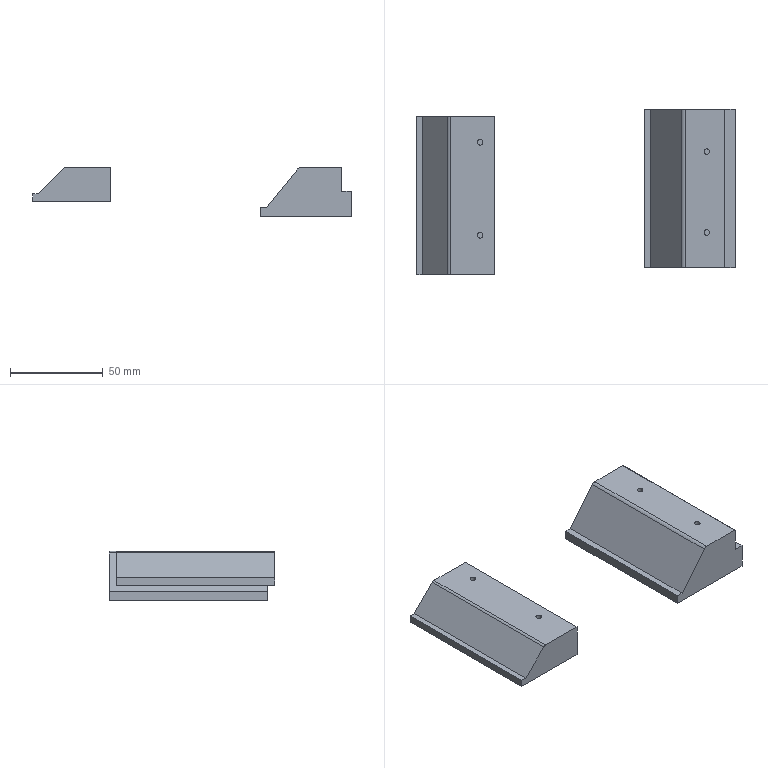NC program | NX | posted with a generic post | part box 171.319 x 88.841 x 26.598 mm
Lines 985 to 3096 of 3096, first 1925 of 2100 lines:
(ZLEVEL_PROFILE_COPY , TOOL : D6R0.5)
N1950 T16 M6
N1952 G54
N1954 G17 G0 G90 X44.509 Y-6.044 S9500 M3
N1956 G43 Z30. H16
N1958 Z1.492
N1960 G94 G1 Z-0.008 F1000.
N1962 X44.022 Y-5.216
N1964 G3 X43.5 Y-4.92 R0.6
N1966 G1 X43.356 Y-4.921 F3000.
N1968 X42.5 Y-5.121
N1970 X-42.5
N1972 X-43.237 Y-4.931
N1974 G2 X-43.39 Y-5.022 R0.113
N1976 G1 X-43.445 Y-5.
N1978 X-43.502 Y-4.969
N1980 X-43.5 Y-5.065 Z-0.017
N1982 G3 X-42.5 Y-5.216 R13.441
N1984 G1 X42.5
N1986 G3 X43.5 Y-5.028 R4.279
N1988 G1 Y-5.14 Z-0.026
N1990 G2 X42.5 Y-5.29 R40.754
N1992 G1 X-42.5
N1994 G2 X-43.5 Y-5.126 R8.99
N1996 G1 Y-5.185 Z-0.035
N1998 G3 X-42.5 Y-5.354 R10.525
N2000 G1 X42.5
N2002 G3 X43.5 Y-5.198 R68.272
N2004 G1 Y-5.242 Z-0.04
N2006 Y-5.252 Z-0.045
N2008 G2 X42.5 Y-5.42 R6.122
N2010 G1 X-42.5
N2012 G2 X-43.5 Y-5.233 R5.293
N2014 G1 Y-5.299 Z-0.06
N2016 G3 X-42.5 Y-5.499 R12.388
N2018 G1 X42.5
N2020 X43.5 Y-5.326
N2022 Y-5.392 Z-0.069
N2024 Y-5.412 Z-0.078
N2026 X42.5 Y-5.579
N2028 X-42.5
N2030 G2 X-43.5 Y-5.378 R2.866
N2032 G1 Y-5.468 Z-0.098
N2034 X-43.376 Y-5.509
N2036 X-42.5 Y-5.659
N2038 X42.5
N2040 X43.5 Y-5.51
N2042 Y-5.548 Z-0.109
N2044 Y-5.585 Z-0.121
N2046 X42.5 Y-5.742
N2048 X-42.5
N2050 X-42.665 Y-5.718
N2052 X-43.529 Y-5.568
N2054 Y-5.602 Z-0.134
N2056 Y-5.658 Z-0.147
N2058 X-42.665 Y-5.813
N2060 X-42.5 Y-5.826
N2062 X42.5
N2064 X43.5 Y-5.67
N2066 Y-5.72 Z-0.161
N2068 Y-5.765 Z-0.175
N2070 X42.5 Y-5.911
N2072 X-42.5
N2074 X-42.665 Y-5.898
N2076 X-43.529 Y-5.758
N2078 X-43.5 Y-5.864 Z-0.207
N2080 X-42.5 Y-5.995
N2082 X42.5
N2084 X43.5 Y-5.866
N2086 Y-5.922 Z-0.224
N2088 Y-5.945 Z-0.242
N2090 X42.5 Y-6.08
N2092 X-42.5
N2094 X-43.5 Y-5.944
N2096 Y-6.008 Z-0.261
N2098 Y-6.031 Z-0.28
N2100 X-43.356 Y-6.034
N2102 X-42.665 Y-6.153
N2104 X-42.5 Y-6.165
N2106 X42.5
N2108 X42.665 Y-6.153
N2110 X43.356 Y-6.035
N2112 X43.5 Y-6.032
N2114 Y-6.092 Z-0.3
N2116 Y-6.126 Z-0.321
N2118 X42.665 Y-6.242
N2120 X42.5 Y-6.249
N2122 X-42.5
N2124 X-42.665 Y-6.242
N2126 X-43.5 Y-6.125
N2128 Y-6.172 Z-0.338
N2130 Y-6.207 Z-0.356
N2132 X-42.665 Y-6.309
N2134 X-42.5 Y-6.317
N2136 X42.5
N2138 X43.5 Y-6.207
N2140 Y-6.251 Z-0.376
N2142 Y-6.289 Z-0.396
N2144 X43.356 Y-6.293
N2146 X42.5 Y-6.389
N2148 X-42.5
N2150 X-42.665 Y-6.383
N2152 X-43.356 Y-6.293
N2154 X-43.5 Y-6.289
N2156 Y-6.342 Z-0.42
N2158 Y-6.387 Z-0.445
N2160 X-43.356 Y-6.389
N2162 X-42.5 Y-6.472
N2164 X42.5
N2166 G2 X43.5 Y-6.387 R24.941
N2168 G1 Y-6.43 Z-0.471
N2170 Y-6.464 Z-0.497
N2172 X43.189 Y-6.47
N2174 X43.011 Y-6.505
N2176 X42.5 Y-6.553
N2178 X-42.5
N2180 G2 X-43.189 Y-6.47 R3.133
N2182 G1 X-43.5 Y-6.464
N2184 Y-6.51 Z-0.524
N2186 Y-6.548 Z-0.551
N2188 X-43.356
N2190 X-42.665 Y-6.625
N2192 X-42.5 Y-6.633
N2194 X42.5
N2196 X42.665 Y-6.625
N2198 X43.356 Y-6.548
N2200 X43.5
N2202 Y-6.588 Z-0.58
N2204 Y-6.625 Z-0.609
N2206 X43.356 Y-6.628
N2208 X42.665 Y-6.706
N2210 X42.5 Y-6.712
N2212 X-42.5
N2214 X-42.665 Y-6.706
N2216 X-43.356 Y-6.628
N2218 X-43.5 Y-6.625
N2220 Y-6.67 Z-0.639
N2222 Y-6.709 Z-0.669
N2224 X-43.356 Y-6.712
N2226 X-42.665 Y-6.781
N2228 X-42.5 Y-6.789
N2230 X42.5
N2232 X42.665 Y-6.781
N2234 X43.356 Y-6.712
N2236 X43.5 Y-6.709
N2238 Y-6.756 Z-0.701
N2240 Y-6.796 Z-0.732
N2242 G3 X42.5 Y-6.864 R11.206
N2244 G1 X-42.5
N2246 X-43.356 Y-6.79
N2248 X-43.5 Y-6.791
N2250 Y-6.834 Z-0.765
N2252 Y-6.868 Z-0.798
N2254 X-43.356 Y-6.87
N2256 X-42.5 Y-6.937
N2258 X42.5
N2260 X43.356 Y-6.872
N2262 X43.5 Y-6.869
N2264 Y-6.907 Z-0.832
N2266 Y-6.936 Z-0.866
N2268 G3 X42.5 Y-7.008 R11.171
N2270 G1 X-42.5
N2272 G3 X-43.5 Y-6.937 R10.417
N2274 G1 Y-6.977 Z-0.901
N2276 Y-7.005 Z-0.936
N2278 X-43.011 Y-7.022
N2280 G3 X-42.5 Y-7.077 R2.311
N2282 G1 X42.5
N2284 G3 X43.011 Y-7.024 R2.413
N2286 G1 X43.5 Y-7.003
N2288 Y-7.043 Z-0.972
N2290 Y-7.072 Z-1.008
N2292 G3 X42.5 Y-7.143 R13.5
N2294 G1 X-42.5
N2296 G3 X-43.5 Y-7.075 R12.04
N2298 G1 Y-7.12 Z-1.045
N2300 Y-7.146 Z-1.083
N2302 G2 X-42.5 Y-7.207 R11.565
N2304 G1 X42.5
N2306 X43.356 Y-7.147
N2308 X43.5 Y-7.142
N2310 Y-7.184 Z-1.121
N2312 Y-7.215 Z-1.159
N2314 X42.5 Y-7.269
N2316 X-42.5
N2318 X-43.356 Y-7.223
N2320 X-43.5 Y-7.22
N2322 Y-7.258 Z-1.198
N2324 Y-7.287 Z-1.237
N2326 G2 X-42.5 Y-7.332 R14.586
N2328 G1 X42.5
N2330 X43.5 Y-7.283
N2332 Y-7.317 Z-1.276
N2334 Y-7.348 Z-1.314
N2336 X42.5 Y-7.395
N2338 X-42.5
N2340 G3 X-43.5 Y-7.353 R13.607
N2342 G1 Y-7.388 Z-1.353
N2344 Y-7.418 Z-1.392
N2346 G2 X-42.5 Y-7.458 R12.751
N2348 G1 X42.5
N2350 X42.665 Y-7.456
N2352 X43.356 Y-7.417
N2354 X43.5 Y-7.413
N2356 Y-7.447 Z-1.431
N2358 Y-7.478 Z-1.47
N2360 X43.356 Y-7.482
N2362 X42.665 Y-7.519
N2364 X42.5 Y-7.521
N2366 X-42.5
N2368 G3 X-43.5 Y-7.483 R11.996
N2370 G1 Y-7.518 Z-1.509
N2372 Y-7.548 Z-1.548
N2374 G2 X-42.5 Y-7.584 R11.325
N2376 G1 X42.5
N2378 X42.665 Y-7.583
N2380 X43.5 Y-7.543
N2382 Y-7.577 Z-1.586
N2384 Y-7.608 Z-1.625
N2386 X43.356 Y-7.613
N2388 X42.665 Y-7.645
N2390 X42.5 Y-7.647
N2392 X-42.5
N2394 G3 X-43.5 Y-7.613 R11.27
N2396 G1 Y-7.648 Z-1.664
N2398 Y-7.678 Z-1.703
N2400 G2 X-42.5 Y-7.71 R12.074
N2402 G1 X42.5
N2404 X42.665 Y-7.708
N2406 X43.5 Y-7.673
N2408 Y-7.708 Z-1.742
N2410 Y-7.739 Z-1.781
N2412 X43.356 Y-7.743
N2414 X42.665 Y-7.771
N2416 X42.5 Y-7.773
N2418 X-42.5
N2420 G3 X-43.5 Y-7.743 R12.986
N2422 G1 Y-7.778 Z-1.82
N2424 Y-7.808 Z-1.858
N2426 G2 X-42.5 Y-7.836 R14.047
N2428 G1 X42.5
N2430 X42.665 Y-7.834
N2432 X43.5 Y-7.804
N2434 Y-7.838 Z-1.897
N2436 Y-7.869 Z-1.936
N2438 X42.665 Y-7.897
N2440 X42.5 Y-7.899
N2442 X-42.5
N2444 G3 X-43.5 Y-7.873 R15.297
N2446 G1 Y-7.909 Z-1.975
N2448 Y-7.938 Z-2.014
N2450 G2 X-42.5 Y-7.962 R16.792
N2452 G1 X42.5
N2454 X42.665 Y-7.96
N2456 X43.5 Y-7.935
N2458 Y-7.968 Z-2.053
N2460 Y-7.999 Z-2.092
N2462 X42.5 Y-8.025
N2464 X-42.5
N2466 X-42.665 Y-8.02
N2468 X-43.5 Y-8.003
N2470 Y-8.039 Z-2.13
N2472 Y-8.068 Z-2.169
N2474 X-42.5 Y-8.087
N2476 X42.5
N2478 X43.5 Y-8.064
N2480 Y-8.098 Z-2.208
N2482 Y-8.129 Z-2.247
N2484 X42.5 Y-8.15
N2486 X-42.5
N2488 X-43.5 Y-8.133
N2490 Y-8.169 Z-2.286
N2492 Y-8.198 Z-2.325
N2494 X-42.5 Y-8.213
N2496 X42.5
N2498 X43.5 Y-8.194
N2500 Y-8.228 Z-2.364
N2502 Y-8.259 Z-2.402
N2504 X42.5 Y-8.276
N2506 X-42.5
N2508 X-42.665 Y-8.272
N2510 X-43.5 Y-8.263
N2512 Y-8.299 Z-2.441
N2514 Y-8.327 Z-2.48
N2516 X-42.665 Y-8.335
N2518 X-42.5 Y-8.339
N2520 X42.5
N2522 X42.665 Y-8.338
N2524 X43.356 Y-8.327
N2526 X43.5 Y-8.323
N2528 Y-8.359 Z-2.519
N2530 Y-8.387 Z-2.558
N2532 X43.356 Y-8.391
N2534 X42.5 Y-8.402
N2536 X-42.5
N2538 X-42.665 Y-8.398
N2540 X-43.5 Y-8.391
N2542 Y-8.428 Z-2.597
N2544 Y-8.455 Z-2.636
N2546 X-42.5 Y-8.465
N2548 X42.5
N2550 X42.665 Y-8.464
N2552 X43.356 Y-8.455
N2554 X43.5 Y-8.451
N2556 Y-8.487 Z-2.674
N2558 Y-8.515 Z-2.713
N2560 X43.356 Y-8.519
N2562 X42.5 Y-8.528
N2564 X-42.5
N2566 X-43.5 Y-8.519
N2568 Y-8.555 Z-2.752
N2570 Y-8.583 Z-2.791
N2572 X-42.5 Y-8.591
N2574 X42.5
N2576 X43.356 Y-8.583
N2578 X43.5 Y-8.579
N2580 Y-8.614 Z-2.83
N2582 Y-8.643 Z-2.869
N2584 X43.356 Y-8.647
N2586 X42.5 Y-8.654
N2588 X-42.5
N2590 X-43.5 Y-8.647
N2592 Y-8.681 Z-2.908
N2594 Y-8.71 Z-2.946
N2596 X-42.665 Y-8.715
N2598 X-42.5 Y-8.717
N2600 X42.5
N2602 X43.356 Y-8.71
N2604 X43.5 Y-8.707
N2606 Y-8.74 Z-2.985
N2608 Y-8.77 Z-3.024
N2610 X43.356 Y-8.774
N2612 X42.5 Y-8.78
N2614 X-42.5
N2616 X-42.665 Y-8.778
N2618 X-43.356 Y-8.776
N2620 X-43.5 Y-8.773
N2622 Y-8.808 Z-3.063
N2624 Y-8.836 Z-3.102
N2626 X-43.356 Y-8.839
N2628 X-42.665 Y-8.841
N2630 X-42.5 Y-8.843
N2632 X42.5
N2634 X43.356 Y-8.837
N2636 X43.5 Y-8.834
N2638 Y-8.867 Z-3.141
N2640 Y-8.897 Z-3.18
N2642 X43.356 Y-8.901
N2644 X42.5 Y-8.906
N2646 X-42.5
N2648 X-42.665 Y-8.904
N2650 X-43.356 Y-8.902
N2652 X-43.5 Y-8.899
N2654 Y-8.934 Z-3.218
N2656 Y-8.963 Z-3.257
N2658 X-43.356 Y-8.966
N2660 X-42.5 Y-8.968
N2662 X42.5
N2664 X43.356 Y-8.964
N2666 X43.5 Y-8.96
N2668 Y-8.994 Z-3.296
N2670 Y-9.024 Z-3.335
N2672 X43.356 Y-9.027
N2674 X42.5 Y-9.031
N2676 X-42.5
N2678 X-43.356 Y-9.029
N2680 X-43.5 Y-9.026
N2682 Y-9.06 Z-3.374
N2684 Y-9.089 Z-3.413
N2686 X-43.356 Y-9.092
N2688 X-42.665 Y-9.093
N2690 X-42.5 Y-9.094
N2692 X42.5
N2694 X43.356 Y-9.091
N2696 X43.5 Y-9.087
N2698 Y-9.121 Z-3.452
N2700 Y-9.151 Z-3.49
N2702 X43.356 Y-9.154
N2704 X42.5 Y-9.157
N2706 X-42.5
N2708 X-42.665 Y-9.156
N2710 X-43.356 Y-9.155
N2712 X-43.5 Y-9.152
N2714 Y-9.187 Z-3.529
N2716 Y-9.215 Z-3.568
N2718 X-43.356 Y-9.218
N2720 X-42.665 Y-9.219
N2722 X-42.5 Y-9.22
N2724 X42.5
N2726 X43.356 Y-9.218
N2728 X43.5 Y-9.214
N2730 Y-9.248 Z-3.607
N2732 Y-9.277 Z-3.646
N2734 X43.356 Y-9.281
N2736 X42.5 Y-9.283
N2738 X-42.5
N2740 X-42.665 Y-9.281
N2742 X-43.356
N2744 X-43.5 Y-9.278
N2746 Y-9.313 Z-3.685
N2748 Y-9.342 Z-3.724
N2750 X-43.356 Y-9.345
N2752 X-42.665
N2754 X-42.5 Y-9.346
N2756 X42.5
N2758 X43.356 Y-9.344
N2760 X43.5 Y-9.341
N2762 Y-9.375 Z-3.762
N2764 Y-9.404 Z-3.801
N2766 X43.356 Y-9.407
N2768 X42.5 Y-9.409
N2770 X-42.5
N2772 X-43.356 Y-9.408
N2774 X-43.5 Y-9.405
N2776 Y-9.439 Z-3.84
N2778 Y-9.468 Z-3.879
N2780 X-43.356 Y-9.471
N2782 X-42.5 Y-9.472
N2784 X42.5
N2786 X43.356 Y-9.47
N2788 X43.5 Y-9.467
N2790 Y-9.502 Z-3.918
N2792 Y-9.53 Z-3.957
N2794 X43.356 Y-9.534
N2796 X42.5 Y-9.535
N2798 X-42.5
N2800 X-43.356 Y-9.534
N2802 X-43.5 Y-9.531
N2804 Y-9.566 Z-3.996
N2806 Y-9.594 Z-4.034
N2808 X-43.356 Y-9.597
N2810 X-42.5 Y-9.598
N2812 X42.5
N2814 X43.356 Y-9.597
N2816 X43.5 Y-9.594
N2818 Y-9.628 Z-4.073
N2820 Y-9.657 Z-4.112
N2822 X43.356 Y-9.66
N2824 X42.5 Y-9.661
N2826 X-42.5
N2828 X-43.356 Y-9.66
N2830 X-43.5 Y-9.657
N2832 Y-9.692 Z-4.151
N2834 Y-9.72 Z-4.19
N2836 X-43.356 Y-9.723
N2838 X-42.5 Y-9.724
N2840 X42.5
N2842 X43.356 Y-9.723
N2844 X43.5 Y-9.72
N2846 Y-9.754 Z-4.229
N2848 Y-9.783 Z-4.268
N2850 X43.356 Y-9.786
N2852 X42.5 Y-9.787
N2854 X-42.5
N2856 X-43.356 Y-9.786
N2858 X-43.5 Y-9.783
N2860 Y-9.818 Z-4.306
N2862 Y-9.846 Z-4.345
N2864 X-43.356 Y-9.849
N2866 X-42.5 Y-9.85
N2868 X42.5
N2870 X43.356 Y-9.849
N2872 X43.5 Y-9.846
N2874 Y-9.88 Z-4.384
N2876 Y-9.909 Z-4.423
N2878 X43.356 Y-9.912
N2880 X42.5
N2882 X-42.5
N2884 X-43.356
N2886 X-43.5 Y-9.909
N2888 Y-9.944 Z-4.462
N2890 Y-9.972 Z-4.501
N2892 X-43.356 Y-9.975
N2894 X-42.5
N2896 X42.5
N2898 X43.356
N2900 X43.5 Y-9.972
N2902 Y-10.006 Z-4.54
N2904 Y-10.035 Z-4.578
N2906 X43.356 Y-10.038
N2908 X42.5
N2910 X-42.5
N2912 X-43.356
N2914 X-43.5 Y-10.035
N2916 Y-10.07 Z-4.617
N2918 Y-10.098 Z-4.656
N2920 X-43.356 Y-10.101
N2922 X-42.5
N2924 X42.5
N2926 X43.356
N2928 X43.5 Y-10.098
N2930 Y-10.132 Z-4.695
N2932 Y-10.161 Z-4.734
N2934 X43.356 Y-10.164
N2936 X42.5
N2938 X-42.5
N2940 X-43.356
N2942 X-43.5 Y-10.161
N2944 Y-10.195 Z-4.773
N2946 Y-10.224 Z-4.812
N2948 X-43.356 Y-10.227
N2950 X-42.5
N2952 X42.5
N2954 X43.356
N2956 X43.5 Y-10.224
N2958 Y-10.258 Z-4.85
N2960 Y-10.287 Z-4.889
N2962 X43.356 Y-10.29
N2964 X42.5
N2966 X-42.5
N2968 X-43.356
N2970 X-43.5 Y-10.287
N2972 Y-10.321 Z-4.928
N2974 Y-10.35 Z-4.967
N2976 X-43.356 Y-10.353
N2978 X-42.5
N2980 X42.5
N2982 X43.356
N2984 X43.5 Y-10.35
N2986 Y-10.384 Z-5.006
N2988 Y-10.413 Z-5.045
N2990 X43.356 Y-10.416
N2992 X42.5
N2994 X-42.5
N2996 X-43.356
N2998 X-43.5 Y-10.413
N3000 Y-10.447 Z-5.084
N3002 Y-10.476 Z-5.122
N3004 X-43.356 Y-10.479
N3006 X-42.5
N3008 X42.5
N3010 X43.356
N3012 X43.5 Y-10.476
N3014 Y-10.51 Z-5.161
N3016 Y-10.539 Z-5.2
N3018 X43.356 Y-10.542
N3020 X42.5
N3022 X-42.5
N3024 X-43.356
N3026 X-43.5 Y-10.539
N3028 Y-10.573 Z-5.239
N3030 Y-10.602 Z-5.278
N3032 X-43.356 Y-10.605
N3034 X-42.5
N3036 X42.5
N3038 X43.356
N3040 X43.5 Y-10.602
N3042 Y-10.636 Z-5.317
N3044 Y-10.665 Z-5.356
N3046 X43.356 Y-10.668
N3048 X42.5
N3050 X-42.5
N3052 X-43.356
N3054 X-43.5 Y-10.665
N3056 Y-10.699 Z-5.394
N3058 Y-10.728 Z-5.433
N3060 X-43.356 Y-10.731
N3062 X-42.5
N3064 X42.5
N3066 X43.356
N3068 X43.5 Y-10.728
N3070 Y-10.762 Z-5.472
N3072 Y-10.79 Z-5.511
N3074 X43.356 Y-10.793
N3076 X42.5 Y-10.794
N3078 X-42.5
N3080 X-43.356 Y-10.793
N3082 X-43.5 Y-10.791
N3084 Y-10.825 Z-5.55
N3086 Y-10.853 Z-5.589
N3088 X-43.356 Y-10.856
N3090 X-42.5
N3092 X42.5
N3094 X43.356
N3096 X43.5 Y-10.853
N3098 Y-10.888 Z-5.628
N3100 Y-10.916 Z-5.666
N3102 X43.356 Y-10.919
N3104 X42.5
N3106 X-42.5
N3108 X-43.356
N3110 X-43.5 Y-10.916
N3112 Y-10.951 Z-5.705
N3114 Y-10.979 Z-5.744
N3116 X-43.356 Y-10.982
N3118 X-42.5
N3120 X42.5
N3122 X43.356
N3124 X43.5 Y-10.979
N3126 Y-11.014 Z-5.783
N3128 Y-11.042 Z-5.822
N3130 X43.356 Y-11.045
N3132 X42.5
N3134 X-42.5
N3136 X-43.356
N3138 X-43.5 Y-11.042
N3140 Y-11.077 Z-5.861
N3142 Y-11.105 Z-5.9
N3144 X-43.356 Y-11.108
N3146 X-42.5
N3148 X42.5
N3150 X43.356
N3152 X43.5 Y-11.105
N3154 Y-11.14 Z-5.938
N3156 Y-11.168 Z-5.977
N3158 X43.356 Y-11.171
N3160 X42.5
N3162 X-42.5
N3164 X-43.356
N3166 X-43.5 Y-11.168
N3168 Y-11.203 Z-6.016
N3170 Y-11.231 Z-6.055
N3172 X-43.356 Y-11.234
N3174 X-42.5
N3176 X42.5
N3178 X43.356
N3180 X43.5 Y-11.231
N3182 Y-11.265 Z-6.094
N3184 Y-11.294 Z-6.133
N3186 X43.356 Y-11.297
N3188 X42.5
N3190 X-42.5
N3192 X-43.356
N3194 X-43.5 Y-11.294
N3196 Y-11.328 Z-6.172
N3198 Y-11.357 Z-6.21
N3200 X-43.356 Y-11.36
N3202 X-42.5
N3204 X42.5
N3206 X43.356
N3208 X43.5 Y-11.357
N3210 Y-11.391 Z-6.249
N3212 Y-11.42 Z-6.288
N3214 X43.356 Y-11.423
N3216 X42.5
N3218 X-42.5
N3220 X-43.356
N3222 X-43.5 Y-11.42
N3224 Y-11.454 Z-6.327
N3226 Y-11.483 Z-6.366
N3228 X-43.356 Y-11.486
N3230 X-42.5
N3232 X42.5
N3234 X43.356
N3236 X43.5 Y-11.483
N3238 Y-11.517 Z-6.405
N3240 Y-11.546 Z-6.444
N3242 X43.356 Y-11.549
N3244 X42.5
N3246 X-42.5
N3248 X-43.356
N3250 X-43.5 Y-11.546
N3252 Y-11.58 Z-6.482
N3254 Y-11.609 Z-6.521
N3256 X-43.356 Y-11.612
N3258 X-42.5
N3260 X42.5
N3262 X43.356
N3264 X43.5 Y-11.609
N3266 Y-11.643 Z-6.56
N3268 Y-11.672 Z-6.599
N3270 X43.356 Y-11.675
N3272 X42.5
N3274 X-42.5
N3276 X-43.356
N3278 X-43.5 Y-11.672
N3280 Y-11.706 Z-6.638
N3282 Y-11.735 Z-6.677
N3284 X-43.356 Y-11.738
N3286 X-42.5
N3288 X42.5
N3290 X43.356
N3292 X43.5 Y-11.735
N3294 Y-11.769 Z-6.716
N3296 Y-11.798 Z-6.754
N3298 X43.356 Y-11.8
N3300 X42.5
N3302 X-42.5
N3304 X-43.356
N3306 X-43.5 Y-11.798
N3308 Y-11.832 Z-6.793
N3310 Y-11.86 Z-6.832
N3312 X-43.356 Y-11.863
N3314 X-42.5
N3316 X42.5
N3318 X43.356
N3320 X43.5 Y-11.86
N3322 Y-11.895 Z-6.871
N3324 Y-11.923 Z-6.91
N3326 X43.356 Y-11.926
N3328 X42.5
N3330 X-42.5
N3332 X-43.356
N3334 X-43.5 Y-11.923
N3336 Y-11.958 Z-6.949
N3338 Y-11.986 Z-6.988
N3340 X-43.356 Y-11.989
N3342 X-42.5
N3344 X42.5
N3346 X43.356
N3348 X43.5 Y-11.986
N3350 Y-12.021 Z-7.026
N3352 Y-12.049 Z-7.065
N3354 X43.356 Y-12.052
N3356 X42.5
N3358 X-42.5
N3360 X-43.356
N3362 X-43.5 Y-12.049
N3364 Y-12.084 Z-7.104
N3366 Y-12.112 Z-7.143
N3368 X-43.356 Y-12.115
N3370 X-42.5
N3372 X42.5
N3374 X43.356
N3376 X43.5 Y-12.112
N3378 Y-12.147 Z-7.182
N3380 Y-12.175 Z-7.221
N3382 X43.356 Y-12.178
N3384 X42.5
N3386 X-42.5
N3388 X-43.356
N3390 X-43.5 Y-12.175
N3392 Y-12.21 Z-7.26
N3394 Y-12.238 Z-7.298
N3396 X-43.356 Y-12.241
N3398 X-42.5
N3400 X42.5
N3402 X43.356
N3404 X43.5 Y-12.238
N3406 Y-12.272 Z-7.337
N3408 Y-12.301 Z-7.376
N3410 X43.356 Y-12.304
N3412 X42.5
N3414 X-42.5
N3416 X-43.356
N3418 X-43.5 Y-12.301
N3420 Y-12.335 Z-7.415
N3422 Y-12.364 Z-7.454
N3424 X-43.356 Y-12.367
N3426 X-42.5
N3428 X42.5
N3430 X43.356
N3432 X43.5 Y-12.364
N3434 Y-12.398 Z-7.493
N3436 Y-12.427 Z-7.532
N3438 X43.356 Y-12.43
N3440 X42.5
N3442 X-42.5
N3444 X-43.356
N3446 X-43.5 Y-12.427
N3448 Y-12.461 Z-7.57
N3450 Y-12.49 Z-7.609
N3452 X-43.356 Y-12.493
N3454 X-42.5
N3456 X42.5
N3458 X43.356
N3460 X43.5 Y-12.49
N3462 Y-12.524 Z-7.648
N3464 Y-12.553 Z-7.687
N3466 X43.356 Y-12.556
N3468 X42.5
N3470 X-42.5
N3472 X-43.356
N3474 X-43.5 Y-12.553
N3476 Y-12.587 Z-7.726
N3478 Y-12.616 Z-7.765
N3480 X-43.356 Y-12.619
N3482 X-42.5
N3484 X42.5
N3486 X43.356
N3488 X43.5 Y-12.616
N3490 Y-12.65 Z-7.804
N3492 Y-12.679 Z-7.842
N3494 X43.356 Y-12.681
N3496 X42.5
N3498 X-42.5
N3500 X-43.356
N3502 X-43.5 Y-12.679
N3504 Y-12.713 Z-7.881
N3506 Y-12.742 Z-7.92
N3508 X-43.356 Y-12.744
N3510 X-42.5
N3512 X42.5
N3514 X43.356
N3516 X43.5 Y-12.741
N3518 Y-12.776 Z-7.959
N3520 Y-12.804 Z-7.998
N3522 X43.356 Y-12.807
N3524 X42.5
N3526 X-42.5
N3528 X-43.356
N3530 X-43.5 Y-12.804
N3532 Y-12.839 Z-8.037
N3534 Y-12.867 Z-8.076
N3536 X-43.356 Y-12.87
N3538 X-42.5
N3540 X42.5
N3542 X43.356
N3544 X43.5 Y-12.867
N3546 Y-12.902 Z-8.114
N3548 Y-12.93 Z-8.153
N3550 X43.356 Y-12.933
N3552 X42.5
N3554 X-42.5
N3556 X-43.356
N3558 X-43.5 Y-12.93
N3560 Y-12.965 Z-8.192
N3562 Y-12.993 Z-8.231
N3564 X-43.356 Y-12.996
N3566 X-42.5
N3568 X42.5
N3570 X43.356
N3572 X43.5 Y-12.993
N3574 Y-13.028 Z-8.27
N3576 Y-13.056 Z-8.309
N3578 X43.356 Y-13.059
N3580 X42.5
N3582 X-42.5
N3584 X-43.356
N3586 X-43.5 Y-13.056
N3588 Y-13.091 Z-8.348
N3590 Y-13.119 Z-8.386
N3592 X-43.356 Y-13.122
N3594 X-42.5
N3596 X42.5
N3598 X43.356
N3600 X43.5 Y-13.119
N3602 Y-13.153 Z-8.425
N3604 Y-13.182 Z-8.464
N3606 X43.356 Y-13.185
N3608 X42.5
N3610 X-42.5
N3612 X-43.356
N3614 X-43.5 Y-13.182
N3616 Y-13.216 Z-8.503
N3618 Y-13.245 Z-8.542
N3620 X-43.356 Y-13.248
N3622 X-42.5
N3624 X42.5
N3626 X43.356
N3628 X43.5 Y-13.245
N3630 Y-13.279 Z-8.581
N3632 Y-13.308 Z-8.62
N3634 X43.356 Y-13.311
N3636 X42.5
N3638 X-42.5
N3640 X-43.356
N3642 X-43.5 Y-13.308
N3644 Y-13.342 Z-8.658
N3646 Y-13.371 Z-8.697
N3648 X-43.356 Y-13.374
N3650 X-42.5
N3652 X42.5
N3654 X43.356
N3656 X43.5 Y-13.371
N3658 Y-13.405 Z-8.736
N3660 Y-13.434 Z-8.775
N3662 X43.356 Y-13.437
N3664 X42.5
N3666 X-42.5
N3668 X-43.356
N3670 X-43.5 Y-13.434
N3672 Y-13.468 Z-8.814
N3674 Y-13.497 Z-8.853
N3676 X-43.356 Y-13.5
N3678 X-42.5
N3680 X42.5
N3682 X43.356
N3684 X43.5 Y-13.497
N3686 Y-13.531 Z-8.892
N3688 Y-13.56 Z-8.93
N3690 X43.356 Y-13.563
N3692 X42.5
N3694 X-42.5
N3696 X-43.356
N3698 X-43.5 Y-13.56
N3700 Y-13.594 Z-8.969
N3702 Y-13.623 Z-9.008
N3704 X-43.356 Y-13.625
N3706 X-42.5
N3708 X42.5
N3710 X43.356
N3712 X43.5 Y-13.623
N3714 Y-13.657 Z-9.047
N3716 Y-13.685 Z-9.086
N3718 X43.356 Y-13.688
N3720 X42.5
N3722 X-42.5
N3724 X-43.356
N3726 X-43.5 Y-13.685
N3728 Y-13.72 Z-9.125
N3730 Y-13.748 Z-9.164
N3732 X-43.356 Y-13.751
N3734 X-42.5
N3736 X42.5
N3738 X43.356
N3740 X43.5 Y-13.748
N3742 Y-13.783 Z-9.202
N3744 Y-13.811 Z-9.241
N3746 X43.356 Y-13.814
N3748 X42.5
N3750 X-42.5
N3752 X-43.356
N3754 X-43.5 Y-13.811
N3756 Y-13.846 Z-9.28
N3758 Y-13.874 Z-9.319
N3760 X-43.356 Y-13.877
N3762 X42.5
N3764 X43.356
N3766 X43.5 Y-13.874
N3768 Y-13.909 Z-9.358
N3770 Y-13.937 Z-9.397
N3772 X43.356 Y-13.94
N3774 X42.5
N3776 X-43.356
N3778 X-43.5 Y-13.937
N3780 Y-13.972 Z-9.436
N3782 Y-14. Z-9.474
N3784 X-43.356 Y-14.003
N3786 X42.5
N3788 X43.356
N3790 X43.5 Y-14.
N3792 Y-14.035 Z-9.513
N3794 Y-14.063 Z-9.552
N3796 X43.356 Y-14.066
N3798 X42.5
N3800 X-43.356
N3802 X-43.5 Y-14.063
N3804 Y-14.097 Z-9.591
N3806 Y-14.126 Z-9.63
N3808 X-43.356 Y-14.129
N3810 X43.356
N3812 X43.5 Y-14.126
N3814 Y-14.16 Z-9.669
N3816 Y-14.189 Z-9.708
N3818 X43.356 Y-14.192
N3820 X-43.356
N3822 X-43.5 Y-14.189
N3824 Y-14.223 Z-9.746
N3826 Y-14.252 Z-9.785
N3828 X-43.356 Y-14.255
N3830 X43.356
N3832 X43.5 Y-14.252
N3834 Y-14.286 Z-9.824
N3836 Y-14.315 Z-9.863
N3838 X43.356 Y-14.318
N3840 X-43.356
N3842 X-43.5 Y-14.315
N3844 Y-14.349 Z-9.902
N3846 Y-14.378 Z-9.941
N3848 X-43.356 Y-14.381
N3850 X43.356
N3852 X43.5 Y-14.378
N3854 Y-14.412 Z-9.98
N3856 Y-14.441 Z-10.018
N3858 X43.356 Y-14.444
N3860 X-43.356
N3862 X-43.5 Y-14.441
N3864 Y-14.475 Z-10.057
N3866 Y-14.504 Z-10.096
N3868 X-43.356 Y-14.507
N3870 X43.356
N3872 X43.5 Y-14.504
N3874 Y-14.538 Z-10.135
N3876 Y-14.567 Z-10.174
N3878 X43.356 Y-14.569
N3880 X-43.356
N3882 X-43.5 Y-14.567
N3884 Y-14.601 Z-10.213
N3886 Y-14.629 Z-10.252
N3888 X-43.356 Y-14.632
N3890 X43.356
N3892 X43.5 Y-14.629
N3894 Y-14.664 Z-10.29
N3896 Y-14.692 Z-10.329
N3898 X43.356 Y-14.695
N3900 X-43.356
N3902 X-43.5 Y-14.692
N3904 Y-14.727 Z-10.368
N3906 Y-14.755 Z-10.407
N3908 X-43.356 Y-14.758
N3910 X43.356
N3912 X43.5 Y-14.755
N3914 Y-14.79 Z-10.446
N3916 Y-14.818 Z-10.485
N3918 X43.356 Y-14.821
N3920 X-43.356
N3922 X-43.5 Y-14.818
N3924 Y-14.853 Z-10.524
N3926 Y-14.881 Z-10.562
N3928 X-43.356 Y-14.884
N3930 X43.356
N3932 X43.5 Y-14.881
N3934 Y-14.916 Z-10.601
N3936 Y-14.944 Z-10.64
N3938 X43.356 Y-14.947
N3940 X-43.356
N3942 X-43.5 Y-14.944
N3944 Y-14.979 Z-10.679
N3946 Y-15.007 Z-10.718
N3948 X-43.356 Y-15.01
N3950 X43.356
N3952 X43.5 Y-15.007
N3954 Y-15.041 Z-10.757
N3956 Y-15.07 Z-10.796
N3958 X43.356 Y-15.073
N3960 X-43.356
N3962 X-43.5 Y-15.07
N3964 Y-15.104 Z-10.834
N3966 Y-15.133 Z-10.873
N3968 X-43.356 Y-15.136
N3970 X43.356
N3972 X43.5 Y-15.133
N3974 Y-15.167 Z-10.912
N3976 Y-15.196 Z-10.951
N3978 X43.356 Y-15.199
N3980 X-43.356
N3982 X-43.5 Y-15.196
N3984 Y-15.23 Z-10.99
N3986 Y-15.259 Z-11.029
N3988 X-43.356 Y-15.262
N3990 X43.356
N3992 X43.5 Y-15.259
N3994 Y-15.293 Z-11.068
N3996 Y-15.322 Z-11.106
N3998 X43.356 Y-15.325
N4000 X-43.356
N4002 X-43.5 Y-15.322
N4004 Y-15.356 Z-11.145
N4006 Y-15.385 Z-11.184
N4008 X-43.356 Y-15.388
N4010 X43.356
N4012 X43.5 Y-15.385
N4014 Y-15.419 Z-11.223
N4016 Y-15.448 Z-11.262
N4018 X43.356 Y-15.451
N4020 X-43.356
N4022 X-43.5 Y-15.448
N4024 Y-15.482 Z-11.301
N4026 Y-15.511 Z-11.34
N4028 X-43.356 Y-15.513
N4030 X43.356
N4032 X43.5 Y-15.511
N4034 Y-15.545 Z-11.378
N4036 Y-15.573 Z-11.417
N4038 X43.356 Y-15.576
N4040 X-43.356
N4042 X-43.5 Y-15.573
N4044 Y-15.608 Z-11.456
N4046 Y-15.636 Z-11.495
N4048 X-43.356 Y-15.639
N4050 X43.356
N4052 X43.5 Y-15.636
N4054 Y-15.671 Z-11.534
N4056 Y-15.699 Z-11.573
N4058 X43.356 Y-15.702
N4060 X-43.356
N4062 X-43.5 Y-15.699
N4064 Y-15.734 Z-11.612
N4066 Y-15.762 Z-11.65
N4068 X-43.356 Y-15.765
N4070 X43.356
N4072 X43.5 Y-15.762
N4074 Y-15.797 Z-11.689
N4076 Y-15.825 Z-11.728
N4078 X43.356 Y-15.828
N4080 X-43.356
N4082 X-43.5 Y-15.825
N4084 Y-15.86 Z-11.767
N4086 Y-15.888 Z-11.806
N4088 X-43.356 Y-15.891
N4090 X43.356
N4092 X43.5 Y-15.888
N4094 Y-15.923 Z-11.845
N4096 Y-15.951 Z-11.884
N4098 X43.356 Y-15.954
N4100 X-43.356
N4102 X-43.5 Y-15.951
N4104 Y-15.985 Z-11.922
N4106 Y-16.014 Z-11.961
N4108 X-43.356 Y-16.017
N4110 X43.356
N4112 X43.5 Y-16.014
N4114 Y-16.048 Z-12.
N4116 Y-16.077 Z-12.039
N4118 X43.356 Y-16.08
N4120 X-43.356
N4122 X-43.5 Y-16.077
N4124 Y-16.111 Z-12.078
N4126 Y-16.14 Z-12.117
N4128 X-43.356 Y-16.143
N4130 X43.356
N4132 X43.5 Y-16.14
N4134 Y-16.174 Z-12.156
N4136 Y-16.203 Z-12.194
N4138 X43.356 Y-16.206
N4140 X-43.356
N4142 X-43.5 Y-16.203
N4144 Y-16.237 Z-12.233
N4146 Y-16.266 Z-12.272
N4148 X-43.356 Y-16.269
N4150 X43.356
N4152 X43.5 Y-16.266
N4154 Y-16.3 Z-12.311
N4156 Y-16.329 Z-12.35
N4158 X43.356 Y-16.332
N4160 X-43.356
N4162 X-43.5 Y-16.329
N4164 Y-16.363 Z-12.389
N4166 Y-16.392 Z-12.428
N4168 X-43.356 Y-16.395
N4170 X43.356
N4172 X43.5 Y-16.392
N4174 Y-16.426 Z-12.466
N4176 Y-16.455 Z-12.505
N4178 X43.356 Y-16.457
N4180 X-43.356
N4182 X-43.5 Y-16.455
N4184 Y-16.489 Z-12.544
N4186 Y-16.517 Z-12.583
N4188 X-43.356 Y-16.52
N4190 X43.356
N4192 X43.5 Y-16.517
N4194 Y-16.552 Z-12.622
N4196 Y-16.58 Z-12.661
N4198 X43.356 Y-16.583
N4200 X-43.356
N4202 X-43.5 Y-16.58
N4204 Y-16.615 Z-12.7
N4206 Y-16.643 Z-12.738
N4208 X-43.356 Y-16.646
N4210 X43.356
N4212 X43.5 Y-16.643
N4214 Y-16.678 Z-12.777
N4216 Y-16.706 Z-12.816
N4218 X43.356 Y-16.709
N4220 X-43.356
N4222 X-43.5 Y-16.706
N4224 Y-16.741 Z-12.855
N4226 Y-16.769 Z-12.894
N4228 X-43.356 Y-16.772
N4230 X43.356
N4232 X43.5 Y-16.769
N4234 Y-16.804 Z-12.933
N4236 Y-16.832 Z-12.972
N4238 X43.356 Y-16.835
N4240 X-43.356
N4242 X-43.5 Y-16.832
N4244 Y-16.866 Z-13.01
N4246 Y-16.895 Z-13.049
N4248 X-43.356 Y-16.898
N4250 X43.356
N4252 X43.5 Y-16.895
N4254 Y-16.929 Z-13.088
N4256 Y-16.958 Z-13.127
N4258 X43.356 Y-16.961
N4260 X-43.356
N4262 X-43.5 Y-16.958
N4264 Y-16.992 Z-13.166
N4266 Y-17.021 Z-13.205
N4268 X-43.356 Y-17.024
N4270 X43.356
N4272 X43.5 Y-17.021
N4274 Y-17.055 Z-13.244
N4276 Y-17.084 Z-13.282
N4278 X43.356 Y-17.087
N4280 X-43.356
N4282 X-43.5 Y-17.084
N4284 Y-17.118 Z-13.321
N4286 Y-17.147 Z-13.36
N4288 X-43.356 Y-17.15
N4290 X43.356
N4292 X43.5 Y-17.147
N4294 Y-17.181 Z-13.399
N4296 Y-17.21 Z-13.438
N4298 X43.356 Y-17.213
N4300 X-43.356
N4302 X-43.5 Y-17.21
N4304 Y-17.244 Z-13.477
N4306 Y-17.273 Z-13.516
N4308 X-43.356 Y-17.276
N4310 X43.356
N4312 X43.5 Y-17.273
N4314 Y-17.307 Z-13.554
N4316 Y-17.336 Z-13.593
N4318 X43.356 Y-17.338
N4320 X-43.356
N4322 X-43.5 Y-17.336
N4324 Y-17.37 Z-13.632
N4326 Y-17.398 Z-13.671
N4328 X-43.356 Y-17.401
N4330 X43.356
N4332 X43.5 Y-17.398
N4334 Y-17.433 Z-13.71
N4336 Y-17.461 Z-13.749
N4338 X43.356 Y-17.464
N4340 X-43.356
N4342 X-43.5 Y-17.461
N4344 Y-17.496 Z-13.788
N4346 Y-17.524 Z-13.826
N4348 X-43.356 Y-17.527
N4350 X43.356
N4352 X43.5 Y-17.524
N4354 Y-17.559 Z-13.865
N4356 Y-17.587 Z-13.904
N4358 X43.356 Y-17.59
N4360 X-43.356
N4362 X-43.5 Y-17.587
N4364 Y-17.622 Z-13.943
N4366 Y-17.65 Z-13.982
N4368 X-43.356 Y-17.653
N4370 X43.356
N4372 X43.5 Y-17.65
N4374 Y-17.685 Z-14.021
N4376 Y-17.713 Z-14.06
N4378 X43.356 Y-17.716
N4380 X-43.356
N4382 X-43.5 Y-17.713
N4384 Y-17.748 Z-14.098
N4386 Y-17.776 Z-14.137
N4388 X-43.356 Y-17.779
N4390 X43.356
N4392 X43.5 Y-17.776
N4394 Y-17.81 Z-14.176
N4396 Y-17.839 Z-14.215
N4398 X43.356 Y-17.842
N4400 X-43.356
N4402 X-43.5 Y-17.839
N4404 Y-17.873 Z-14.254
N4406 Y-17.902 Z-14.293
N4408 X-43.356 Y-17.905
N4410 X43.356
N4412 X43.5 Y-17.902
N4414 Y-17.936 Z-14.332
N4416 Y-17.965 Z-14.37
N4418 X43.356 Y-17.968
N4420 X-43.356
N4422 X-43.5 Y-17.965
N4424 Y-17.999 Z-14.409
N4426 Y-18.028 Z-14.448
N4428 X-43.356 Y-18.031
N4430 X43.356
N4432 X43.5 Y-18.028
N4434 Y-18.062 Z-14.487
N4436 Y-18.091 Z-14.526
N4438 X43.356 Y-18.094
N4440 X-43.356
N4442 X-43.5 Y-18.091
N4444 Y-18.125 Z-14.565
N4446 Y-18.154 Z-14.604
N4448 X-43.356 Y-18.157
N4450 X43.356
N4452 X43.5 Y-18.154
N4454 Y-18.188 Z-14.642
N4456 Y-18.217 Z-14.681
N4458 X43.356 Y-18.22
N4460 X-43.356
N4462 X-43.5 Y-18.217
N4464 Y-18.251 Z-14.72
N4466 Y-18.28 Z-14.759
N4468 X-43.356 Y-18.282
N4470 X43.356
N4472 X43.5 Y-18.28
N4474 Y-18.314 Z-14.798
N4476 Y-18.342 Z-14.837
N4478 X43.356 Y-18.345
N4480 X-43.356
N4482 X-43.499 Y-18.342
N4484 Y-18.377 Z-14.876
N4486 Y-18.405 Z-14.914
N4488 X-43.356 Y-18.408
N4490 X43.356
N4492 X43.499 Y-18.405
N4494 Y-18.44 Z-14.953
N4496 Y-18.468 Z-14.992
N4498 X43.356 Y-18.471
N4500 X-43.356
N4502 X-43.499 Y-18.468
N4504 Y-18.503 Z-15.031
N4506 Y-18.531 Z-15.07
N4508 X-43.356 Y-18.534
N4510 X43.356
N4512 X43.499 Y-18.531
N4514 Y-18.566 Z-15.109
N4516 Y-18.594 Z-15.148
N4518 X43.356 Y-18.597
N4520 X-43.356
N4522 X-43.499 Y-18.594
N4524 Y-18.629 Z-15.186
N4526 Y-18.657 Z-15.225
N4528 X-43.356 Y-18.66
N4530 X43.356
N4532 X43.499 Y-18.657
N4534 Y-18.692 Z-15.264
N4536 Y-18.72 Z-15.303
N4538 X43.356 Y-18.723
N4540 X-43.356
N4542 X-43.499 Y-18.72
N4544 Y-18.754 Z-15.342
N4546 Y-18.783 Z-15.381
N4548 X-43.356 Y-18.786
N4550 X43.356
N4552 X43.499 Y-18.783
N4554 Y-18.817 Z-15.42
N4556 Y-18.846 Z-15.458
N4558 X43.356 Y-18.849
N4560 X-43.356
N4562 X-43.499 Y-18.846
N4564 Y-18.88 Z-15.497
N4566 Y-18.909 Z-15.536
N4568 X-43.356 Y-18.912
N4570 X42.5
N4572 X43.356
N4574 X43.499 Y-18.909
N4576 Y-18.943 Z-15.575
N4578 Y-18.972 Z-15.614
N4580 X43.356 Y-18.975
N4582 X42.5
N4584 X-43.356
N4586 X-43.499 Y-18.972
N4588 Y-19.006 Z-15.653
N4590 Y-19.035 Z-15.692
N4592 X-43.356 Y-19.038
N4594 X42.5
N4596 X43.356
N4598 X43.499 Y-19.035
N4600 Y-19.069 Z-15.73
N4602 Y-19.098 Z-15.769
N4604 X43.356 Y-19.101
N4606 X42.5
N4608 X-43.356
N4610 X-43.499 Y-19.098
N4612 Y-19.132 Z-15.808
N4614 Y-19.161 Z-15.847
N4616 X-43.356 Y-19.164
N4618 X42.5
N4620 X43.356
N4622 X43.499 Y-19.161
N4624 Y-19.195 Z-15.886
N4626 Y-19.224 Z-15.925
N4628 X43.356 Y-19.226
N4630 X42.5
N4632 X-43.356
N4634 X-43.499 Y-19.224
N4636 Y-19.258 Z-15.964
N4638 Y-19.286 Z-16.002
N4640 X-43.356 Y-19.289
N4642 X42.5
N4644 X43.356
N4646 X43.499 Y-19.286
N4648 Y-19.321 Z-16.041
N4650 Y-19.349 Z-16.08
N4652 X43.356 Y-19.352
N4654 X42.5
N4656 X-43.356
N4658 X-43.499 Y-19.349
N4660 Y-19.384 Z-16.119
N4662 Y-19.412 Z-16.158
N4664 X-43.356 Y-19.415
N4666 X42.5
N4668 X43.356
N4670 X43.499 Y-19.412
N4672 Y-19.447 Z-16.197
N4674 Y-19.475 Z-16.236
N4676 X43.356 Y-19.478
N4678 X42.5
N4680 X-43.356
N4682 X-43.499 Y-19.475
N4684 Y-19.51 Z-16.274
N4686 Y-19.538 Z-16.313
N4688 X-43.356 Y-19.541
N4690 X42.5
N4692 X43.356
N4694 X43.499 Y-19.538
N4696 Y-19.573 Z-16.352
N4698 Y-19.601 Z-16.391
N4700 X43.356 Y-19.604
N4702 X42.5
N4704 X-43.356
N4706 X-43.499 Y-19.601
N4708 Y-19.636 Z-16.43
N4710 Y-19.664 Z-16.469
N4712 X-43.356 Y-19.667
N4714 X42.5
N4716 X43.356
N4718 X43.499 Y-19.664
N4720 X43.498 Y-19.698 Z-16.508
N4722 Y-19.727 Z-16.546
N4724 X43.356 Y-19.73
N4726 X42.5
N4728 X-43.356
N4730 X-43.498 Y-19.727
N4732 Y-19.761 Z-16.585
N4734 Y-19.79 Z-16.624
N4736 X-43.356 Y-19.793
N4738 X42.5
N4740 X43.356
N4742 X43.498 Y-19.79
N4744 Y-19.824 Z-16.663
N4746 Y-19.853 Z-16.702
N4748 X43.356 Y-19.856
N4750 X42.5
N4752 X-43.356
N4754 X-43.498 Y-19.853
N4756 Y-19.887 Z-16.741
N4758 Y-19.916 Z-16.78
N4760 X-43.356 Y-19.919
N4762 X42.5
N4764 X43.356
N4766 X43.498 Y-19.916
N4768 Y-19.95 Z-16.818
N4770 Y-19.979 Z-16.857
N4772 X43.356 Y-19.982
N4774 X42.5
N4776 X-43.356
N4778 X-43.498 Y-19.979
N4780 Y-20.013 Z-16.896
N4782 Y-20.042 Z-16.935
N4784 X-43.356 Y-20.045
N4786 X42.5
N4788 X43.356
N4790 X43.498 Y-20.042
N4792 Y-20.076 Z-16.974
N4794 Y-20.105 Z-17.013
N4796 X43.356 Y-20.108
N4798 X42.5
N4800 X-43.356
N4802 X-43.498 Y-20.105
N4804 Y-20.139 Z-17.052
N4806 Y-20.167 Z-17.09
N4808 X-43.356 Y-20.17
N4810 X42.5
N4812 X43.356
N4814 X43.498 Y-20.167
N4816 Y-20.202 Z-17.129
N4818 Y-20.23 Z-17.168
N4820 X43.356 Y-20.233
N4822 X42.5
N4824 X-43.356
N4826 X-43.498 Y-20.23
N4828 Y-20.265 Z-17.207
N4830 Y-20.293 Z-17.246
N4832 X-43.356 Y-20.296
N4834 X42.5
N4836 X43.356
N4838 X43.498 Y-20.293
N4840 Y-20.328 Z-17.285
N4842 Y-20.356 Z-17.324
N4844 X43.356 Y-20.359
N4846 X42.5
N4848 X-43.356
N4850 X-43.498 Y-20.356
N4852 X-43.497 Y-20.391 Z-17.362
N4854 Y-20.419 Z-17.401
N4856 X-43.356 Y-20.422
N4858 X42.5
N4860 X43.356
N4862 X43.497 Y-20.419
N4864 Y-20.454 Z-17.44
N4866 Y-20.482 Z-17.479
N4868 X43.356 Y-20.485
N4870 X42.5
N4872 X-43.356
N4874 X-43.497 Y-20.482
N4876 Y-20.517 Z-17.518
N4878 Y-20.545 Z-17.557
N4880 X-43.356 Y-20.548
N4882 X42.5
N4884 X43.356
N4886 X43.497 Y-20.545
N4888 Y-20.579 Z-17.596
N4890 Y-20.608 Z-17.634
N4892 X43.356 Y-20.611
N4894 X42.5
N4896 X-43.356
N4898 X-43.497 Y-20.608
N4900 Y-20.642 Z-17.673
N4902 Y-20.671 Z-17.712
N4904 X-43.356 Y-20.674
N4906 X42.5
N4908 X43.356
N4910 X43.496 Y-20.671
N4912 Y-20.705 Z-17.751
N4914 Y-20.734 Z-17.79
N4916 X43.356 Y-20.737
N4918 X42.5
N4920 X-43.356
N4922 X-43.496 Y-20.734
N4924 Y-20.768 Z-17.829
N4926 Y-20.797 Z-17.868
N4928 X-43.356 Y-20.8
N4930 X42.5
N4932 X43.356
N4934 X43.496 Y-20.797
N4936 Y-20.831 Z-17.906
N4938 Y-20.86 Z-17.945
N4940 X43.356 Y-20.863
N4942 X42.5
N4944 X-43.356
N4946 X-43.496 Y-20.86
N4948 Y-20.894 Z-17.984
N4950 Y-20.923 Z-18.023
N4952 X-43.356 Y-20.926
N4954 X42.5
N4956 X43.356
N4958 X43.496 Y-20.923
N4960 Y-20.957 Z-18.062
N4962 X43.495 Y-20.986 Z-18.101
N4964 X43.356 Y-20.989
N4966 X42.5
N4968 X-43.356
N4970 X-43.495 Y-20.986
N4972 Y-21.02 Z-18.14
N4974 Y-21.049 Z-18.178
N4976 X-43.356 Y-21.051
N4978 X42.5
N4980 X43.356
N4982 X43.495 Y-21.049
N4984 Y-21.083 Z-18.217
N4986 Y-21.111 Z-18.256
N4988 X43.356 Y-21.114
N4990 X42.5
N4992 X-43.356
N4994 X-43.495 Y-21.111
N4996 Y-21.146 Z-18.295
N4998 Y-21.174 Z-18.334
N5000 X-43.356 Y-21.177
N5002 X42.5
N5004 X43.356
N5006 X43.495 Y-21.174
N5008 Y-21.209 Z-18.373
N5010 Y-21.237 Z-18.412
N5012 X43.356 Y-21.24
N5014 X42.5
N5016 X-43.356
N5018 X-43.495 Y-21.237
N5020 Y-21.272 Z-18.45
N5022 X-43.494 Y-21.3 Z-18.489
N5024 X-43.356 Y-21.303
N5026 X42.5
N5028 X43.356
N5030 X43.495 Y-21.3
N5032 X43.494 Y-21.335 Z-18.528
N5034 Y-21.363 Z-18.567
N5036 X43.356 Y-21.366
N5038 X42.5
N5040 X-43.356
N5042 X-43.494 Y-21.363
N5044 Y-21.398 Z-18.606
N5046 Y-21.426 Z-18.645
N5048 X-43.356 Y-21.429
N5050 X42.5
N5052 X43.356
N5054 X43.494 Y-21.426
N5056 Y-21.461 Z-18.684
N5058 Y-21.489 Z-18.722
N5060 X43.356 Y-21.492
N5062 X42.5
N5064 X-43.356
N5066 X-43.494 Y-21.489
N5068 Y-21.523 Z-18.761
N5070 X-43.493 Y-21.552 Z-18.8
N5072 X-43.356 Y-21.555
N5074 X42.5
N5076 X43.356
N5078 X43.493 Y-21.552
N5080 Y-21.586 Z-18.839
N5082 Y-21.615 Z-18.878
N5084 X43.356 Y-21.618
N5086 X42.5
N5088 X-43.356
N5090 X-43.493 Y-21.615
N5092 Y-21.649 Z-18.917
N5094 Y-21.678 Z-18.956
N5096 X-43.356 Y-21.681
N5098 X42.5
N5100 X43.356
N5102 X43.493 Y-21.678
N5104 Y-21.712 Z-18.994
N5106 X43.492 Y-21.741 Z-19.033
N5108 X43.356 Y-21.744
N5110 X42.5
N5112 X-43.356
N5114 X-43.493 Y-21.741
N5116 X-43.492 Y-21.775 Z-19.072
N5118 Y-21.804 Z-19.111
N5120 X-43.356 Y-21.807
N5122 X42.5
N5124 X43.356
N5126 X43.492 Y-21.804
N5128 Y-21.838 Z-19.15
N5130 Y-21.867 Z-19.189
N5132 X43.356 Y-21.87
N5134 X42.5
N5136 X-43.356
N5138 X-43.492 Y-21.867
N5140 Y-21.901 Z-19.228
N5142 X-43.491 Y-21.93 Z-19.266
N5144 X-43.356 Y-21.933
N5146 X42.5
N5148 X43.356
N5150 X43.491 Y-21.93
N5152 Y-21.964 Z-19.305
N5154 Y-21.992 Z-19.344
N5156 X43.356 Y-21.995
N5158 X42.5
N5160 X-43.356
N5162 X-43.491 Y-21.992
N5164 Y-22.027 Z-19.383
N5166 X-43.49 Y-22.055 Z-19.422
N5168 X-43.356 Y-22.058
N5170 X42.5
N5172 X43.356
N5174 X43.49 Y-22.055
N5176 Y-22.09 Z-19.461
N5178 Y-22.118 Z-19.5
N5180 X43.356 Y-22.121
N5182 X42.5
N5184 X-43.356
N5186 X-43.49 Y-22.118
N5188 Y-22.153 Z-19.538
N5190 Y-22.181 Z-19.577
N5192 X-43.356 Y-22.184
N5194 X42.5
N5196 X43.356
N5198 X43.49 Y-22.181
N5200 X43.489 Y-22.216 Z-19.616
N5202 Y-22.244 Z-19.655
N5204 X43.356 Y-22.247
N5206 X42.5
N5208 X-43.356
N5210 X-43.489 Y-22.244
N5212 Y-22.279 Z-19.694
N5214 Y-22.307 Z-19.733
N5216 X-43.356 Y-22.31
N5218 X42.5
N5220 X43.356
N5222 X43.489 Y-22.307
N5224 Y-22.342 Z-19.772
N5226 X43.488 Y-22.37 Z-19.81
N5228 X43.356 Y-22.373
N5230 X42.5
N5232 X-43.356
N5234 X-43.488 Y-22.37
N5236 Y-22.405 Z-19.849
N5238 Y-22.433 Z-19.888
N5240 X-43.356 Y-22.436
N5242 X42.5
N5244 X43.356
N5246 X43.488 Y-22.433
N5248 Y-22.467 Z-19.927
N5250 Y-22.496 Z-19.966
N5252 X43.356 Y-22.499
N5254 X42.5
N5256 X-43.356
N5258 X-43.488 Y-22.496
N5260 X-43.487 Y-22.53 Z-20.005
N5262 Y-22.559 Z-20.044
N5264 X-43.356 Y-22.562
N5266 X42.5
N5268 X43.356
N5270 X43.487 Y-22.559
N5272 Y-22.593 Z-20.082
N5274 Y-22.622 Z-20.121
N5276 X43.356 Y-22.625
N5278 X42.5
N5280 X-43.356
N5282 X-43.487 Y-22.622
N5284 X-43.486 Y-22.656 Z-20.16
N5286 Y-22.685 Z-20.199
N5288 X-43.356 Y-22.688
N5290 X42.5
N5292 X43.356
N5294 X43.486 Y-22.685
N5296 Y-22.719 Z-20.238
N5298 Y-22.748 Z-20.277
N5300 X43.356 Y-22.751
N5302 X42.5
N5304 X-43.356
N5306 X-43.486 Y-22.748
N5308 Y-22.782 Z-20.316
N5310 X-43.485 Y-22.811 Z-20.354
N5312 X-43.356 Y-22.814
N5314 X42.5
N5316 X43.356
N5318 X43.485 Y-22.811
N5320 Y-22.845 Z-20.393
N5322 Y-22.873 Z-20.432
N5324 X43.356 Y-22.877
N5326 X42.5
N5328 X-43.356
N5330 X-43.485 Y-22.873
N5332 Y-22.908 Z-20.471
N5334 X-43.484 Y-22.936 Z-20.51
N5336 X-43.356 Y-22.939
N5338 X42.5
N5340 X43.356
N5342 X43.484 Y-22.936
N5344 Y-22.971 Z-20.549
N5346 Y-22.999 Z-20.588
N5348 X43.356 Y-23.002
N5350 X42.5
N5352 X-43.356
N5354 X-43.484 Y-22.999
N5356 X-43.483 Y-23.034 Z-20.626
N5358 Y-23.062 Z-20.665
N5360 X-43.356 Y-23.065
N5362 X42.5
N5364 X43.356
N5366 X43.483 Y-23.062
N5368 Y-23.097 Z-20.704
N5370 Y-23.125 Z-20.743
N5372 X43.356 Y-23.128
N5374 X42.5
N5376 X-43.356
N5378 X-43.483 Y-23.125
N5380 X-43.482 Y-23.16 Z-20.782
N5382 Y-23.188 Z-20.821
N5384 X-43.356 Y-23.191
N5386 X42.5
N5388 X43.356
N5390 X43.482 Y-23.188
N5392 Y-23.223 Z-20.86
N5394 Y-23.251 Z-20.898
N5396 X43.356 Y-23.254
N5398 X42.5
N5400 X-43.356
N5402 X-43.482 Y-23.251
N5404 X-43.481 Y-23.286 Z-20.937
N5406 Y-23.314 Z-20.976
N5408 X-43.356 Y-23.317
N5410 X42.5
N5412 X43.356
N5414 X43.481 Y-23.314
N5416 Y-23.349 Z-21.015
N5418 X43.48 Y-23.377 Z-21.054
N5420 X43.356 Y-23.38
N5422 X42.5
N5424 X-43.356
N5426 X-43.48 Y-23.377
N5428 Y-23.411 Z-21.093
N5430 Y-23.44 Z-21.132
N5432 X-43.356 Y-23.443
N5434 X42.5
N5436 X43.356
N5438 X43.48 Y-23.44
N5440 Y-23.474 Z-21.17
N5442 X43.479 Y-23.503 Z-21.209
N5444 X43.356 Y-23.506
N5446 X42.5
N5448 X-43.356
N5450 X-43.479 Y-23.503
N5452 X-43.457 Y-23.566 Z-21.287
N5454 X-43.356 Y-23.569
N5456 X-42.5
N5458 X42.5
N5460 X43.356
N5462 X43.457 Y-23.566
N5464 X43.432 Y-23.63 Z-21.365
N5466 X43.356 Y-23.632
N5468 X42.5
N5470 X-42.5
N5472 X-43.356
N5474 X-43.432 Y-23.63
N5476 X-43.407 Y-23.694 Z-21.443
N5478 X-43.356 Y-23.695
N5480 X-42.5
N5482 X42.5
N5484 X43.356
N5486 X43.407 Y-23.694
N5488 X43.381 Y-23.757 Z-21.52
N5490 X42.5 Y-23.758
N5492 X-42.5
N5494 X-43.381 Y-23.757
N5496 X-43.357 Y-23.819 Z-21.598
N5498 X-42.5
N5500 X42.5
N5502 X43.357
N5504 G2 X43.876 Y-24.119 R0.6
N5506 G1 X44.342 Y-24.927
N5508 Z-20.098
N5510 G0 Z30.
(ZLEVEL_PROFILE_COPY_COPY , TOOL : D6R0.5)
N5512 X-44.415 Y22.534
N5514 Z1.486
N5516 G1 Z-0.014 F1000.
N5518 X-44.006 Y21.759
N5520 G3 X-43.498 Y21.439 R0.6
N5522 G1 X-43.356 Y21.434 F3000.
N5524 X-42.5 Y21.512
N5526 X42.5
N5528 X43.356 Y21.434
N5530 X43.498 Y21.439
N5532 X43.5 Y21.5 Z-0.024
N5534 Y21.525 Z-0.035
N5536 X43.356 Y21.529
N5538 X42.5 Y21.608
N5540 X-42.5
N5542 X-42.665 Y21.588
N5544 X-43.356 Y21.531
N5546 X-43.5 Y21.528
N5548 Y21.583 Z-0.048
N5550 X-43.501 Y21.609 Z-0.061
N5552 X-42.5 Y21.692
N5554 X42.5
N5556 X43.501 Y21.601
N5558 Y21.644 Z-0.078
N5560 Y21.68 Z-0.094
N5562 X42.5 Y21.771
N5564 X-42.5
N5566 X-43.5 Y21.688
N5568 Y21.736 Z-0.115
N5570 Y21.762 Z-0.135
N5572 X-42.665 Y21.84
N5574 X-42.5 Y21.848
N5576 X42.5
N5578 G2 X43.096 Y21.777 R2.53
N5580 G1 X43.501 Y21.752
N5582 X43.5 Y21.802 Z-0.16
N5584 Y21.836 Z-0.184
N5586 X43.356 Y21.84
N5588 X42.5 Y21.924
N5590 X-42.5
N5592 X-43.5 Y21.845
N5594 Y21.885 Z-0.211
N5596 Y21.917 Z-0.238
N5598 X-43.356 Y21.92
N5600 X-42.5 Y21.994
N5602 X42.5
N5604 X43.356 Y21.916
N5606 X43.501 Y21.912
N5608 Y21.96 Z-0.271
N5610 Y22.002 Z-0.303
N5612 X43.356 Y22.004
N5614 X42.5 Y22.064
N5616 X-42.5
N5618 G2 X-43.501 Y22.002 R17.128
N5620 G1 Y22.036 Z-0.34
N5622 Y22.067 Z-0.376
N5624 G3 X-42.5 Y22.128 R17.974
N5626 G1 X42.5
N5628 X43.356 Y22.063
N5630 X43.5 Y22.06
N5632 Y22.101 Z-0.416
N5634 Y22.124 Z-0.455
N5636 X43.011 Y22.14
N5638 G3 X42.5 Y22.185 R3.396
N5640 G1 X-42.5
N5642 G3 X-43.011 Y22.142 R3.881
N5644 G1 X-43.5 Y22.124
N5646 X-43.499 Y22.155 Z-0.498
N5648 X-43.498 Y22.18 Z-0.541
N5650 G3 X-42.5 Y22.235 R14.494
N5652 G1 X42.5
N5654 G3 X43.497 Y22.186 R13.989
N5656 G1 X43.492 Y22.215 Z-0.586
N5658 X43.489 Y22.237 Z-0.631
N5660 G2 X42.5 Y22.276 R14.745
N5662 G1 X-42.5
N5664 X-43.49 Y22.232
N5666 X-43.486 Y22.256 Z-0.677
N5668 X-43.482 Y22.276 Z-0.723
N5670 G3 X-42.5 Y22.307 R78.73
N5672 G1 X42.5
N5674 G3 X43.481 Y22.279 R16.543
N5676 G1 X43.472 Y22.309 Z-0.816
N5678 X42.665 Y22.319
N5680 X42.5 Y22.329
N5682 X-42.5
N5684 X-43.473 Y22.31
N5686 X-43.464 Y22.331 Z-0.908
N5688 X-42.665 Y22.336
N5690 X-42.5 Y22.342
N5692 X42.5
N5694 X42.665 Y22.335
N5696 X43.463 Y22.33
N5698 X43.454 Y22.343 Z-1.
N5700 X-43.455 Y22.344
N5702 G2 X-43.975 Y22.644 R0.6
N5704 G1 X-44.435 Y23.44
N5706 Z0.5
N5708 G0 Z30.
N5710 M5
(HOLE_MILLING_COPY , TOOL : D2)
N5712 T17 M6
N5714 G54
N5716 G17 G0 G90 X-19.75 Y9.206 S9500 M3
N5718 G43 Z30. H17
N5720 Z0.5
N5722 G94 G3 X-19.55 Y9.406 R0.2 F1000.
N5724 X-19.75 Y9.606 R0.2
N5726 X-19.75 Y9.606 Z0.35 I0. J-0.4
N5728 X-19.75 Y9.606 Z0.2 I0. J-0.4
N5730 X-19.75 Y9.606 Z0.05 I0. J-0.4
N5732 X-19.75 Y9.606 Z-0.1 I0. J-0.4
N5734 X-19.75 Y9.606 Z-0.25 I0. J-0.4
N5736 X-19.75 Y9.606 Z-0.4 I0. J-0.4
N5738 X-19.75 Y9.606 Z-0.55 I0. J-0.4
N5740 X-19.75 Y9.606 Z-0.7 I0. J-0.4
N5742 X-19.75 Y9.606 Z-0.85 I0. J-0.4
N5744 X-19.75 Y9.606 Z-1. I0. J-0.4
N5746 X-19.75 Y9.606 Z-1.15 I0. J-0.4
N5748 X-19.75 Y9.606 Z-1.3 I0. J-0.4
N5750 X-19.75 Y9.606 Z-1.45 I0. J-0.4
N5752 X-19.75 Y9.606 Z-1.6 I0. J-0.4
N5754 X-19.75 Y9.606 Z-1.75 I0. J-0.4
N5756 X-19.75 Y9.606 Z-1.9 I0. J-0.4
N5758 X-19.75 Y9.606 Z-2.05 I0. J-0.4
N5760 X-19.75 Y9.606 Z-2.2 I0. J-0.4
N5762 X-19.75 Y9.606 Z-2.35 I0. J-0.4
N5764 X-19.75 Y9.606 Z-2.5 I0. J-0.4
N5766 X-19.75 Y9.606 Z-2.65 I0. J-0.4
N5768 X-19.75 Y9.606 Z-2.8 I0. J-0.4
N5770 X-19.75 Y9.606 Z-2.95 I0. J-0.4
N5772 X-19.75 Y9.606 Z-3.1 I0. J-0.4
N5774 X-19.75 Y9.606 Z-3.25 I0. J-0.4
N5776 X-19.75 Y9.606 Z-3.4 I0. J-0.4
N5778 X-19.75 Y9.606 Z-3.55 I0. J-0.4
N5780 X-19.75 Y9.606 Z-3.7 I0. J-0.4
N5782 X-19.75 Y9.606 Z-3.85 I0. J-0.4
N5784 X-19.75 Y9.606 Z-4. I0. J-0.4
N5786 X-19.75 Y9.606 Z-4.15 I0. J-0.4
N5788 X-19.75 Y9.606 Z-4.3 I0. J-0.4
N5790 X-19.75 Y9.606 Z-4.45 I0. J-0.4
N5792 X-19.75 Y9.606 Z-4.6 I0. J-0.4